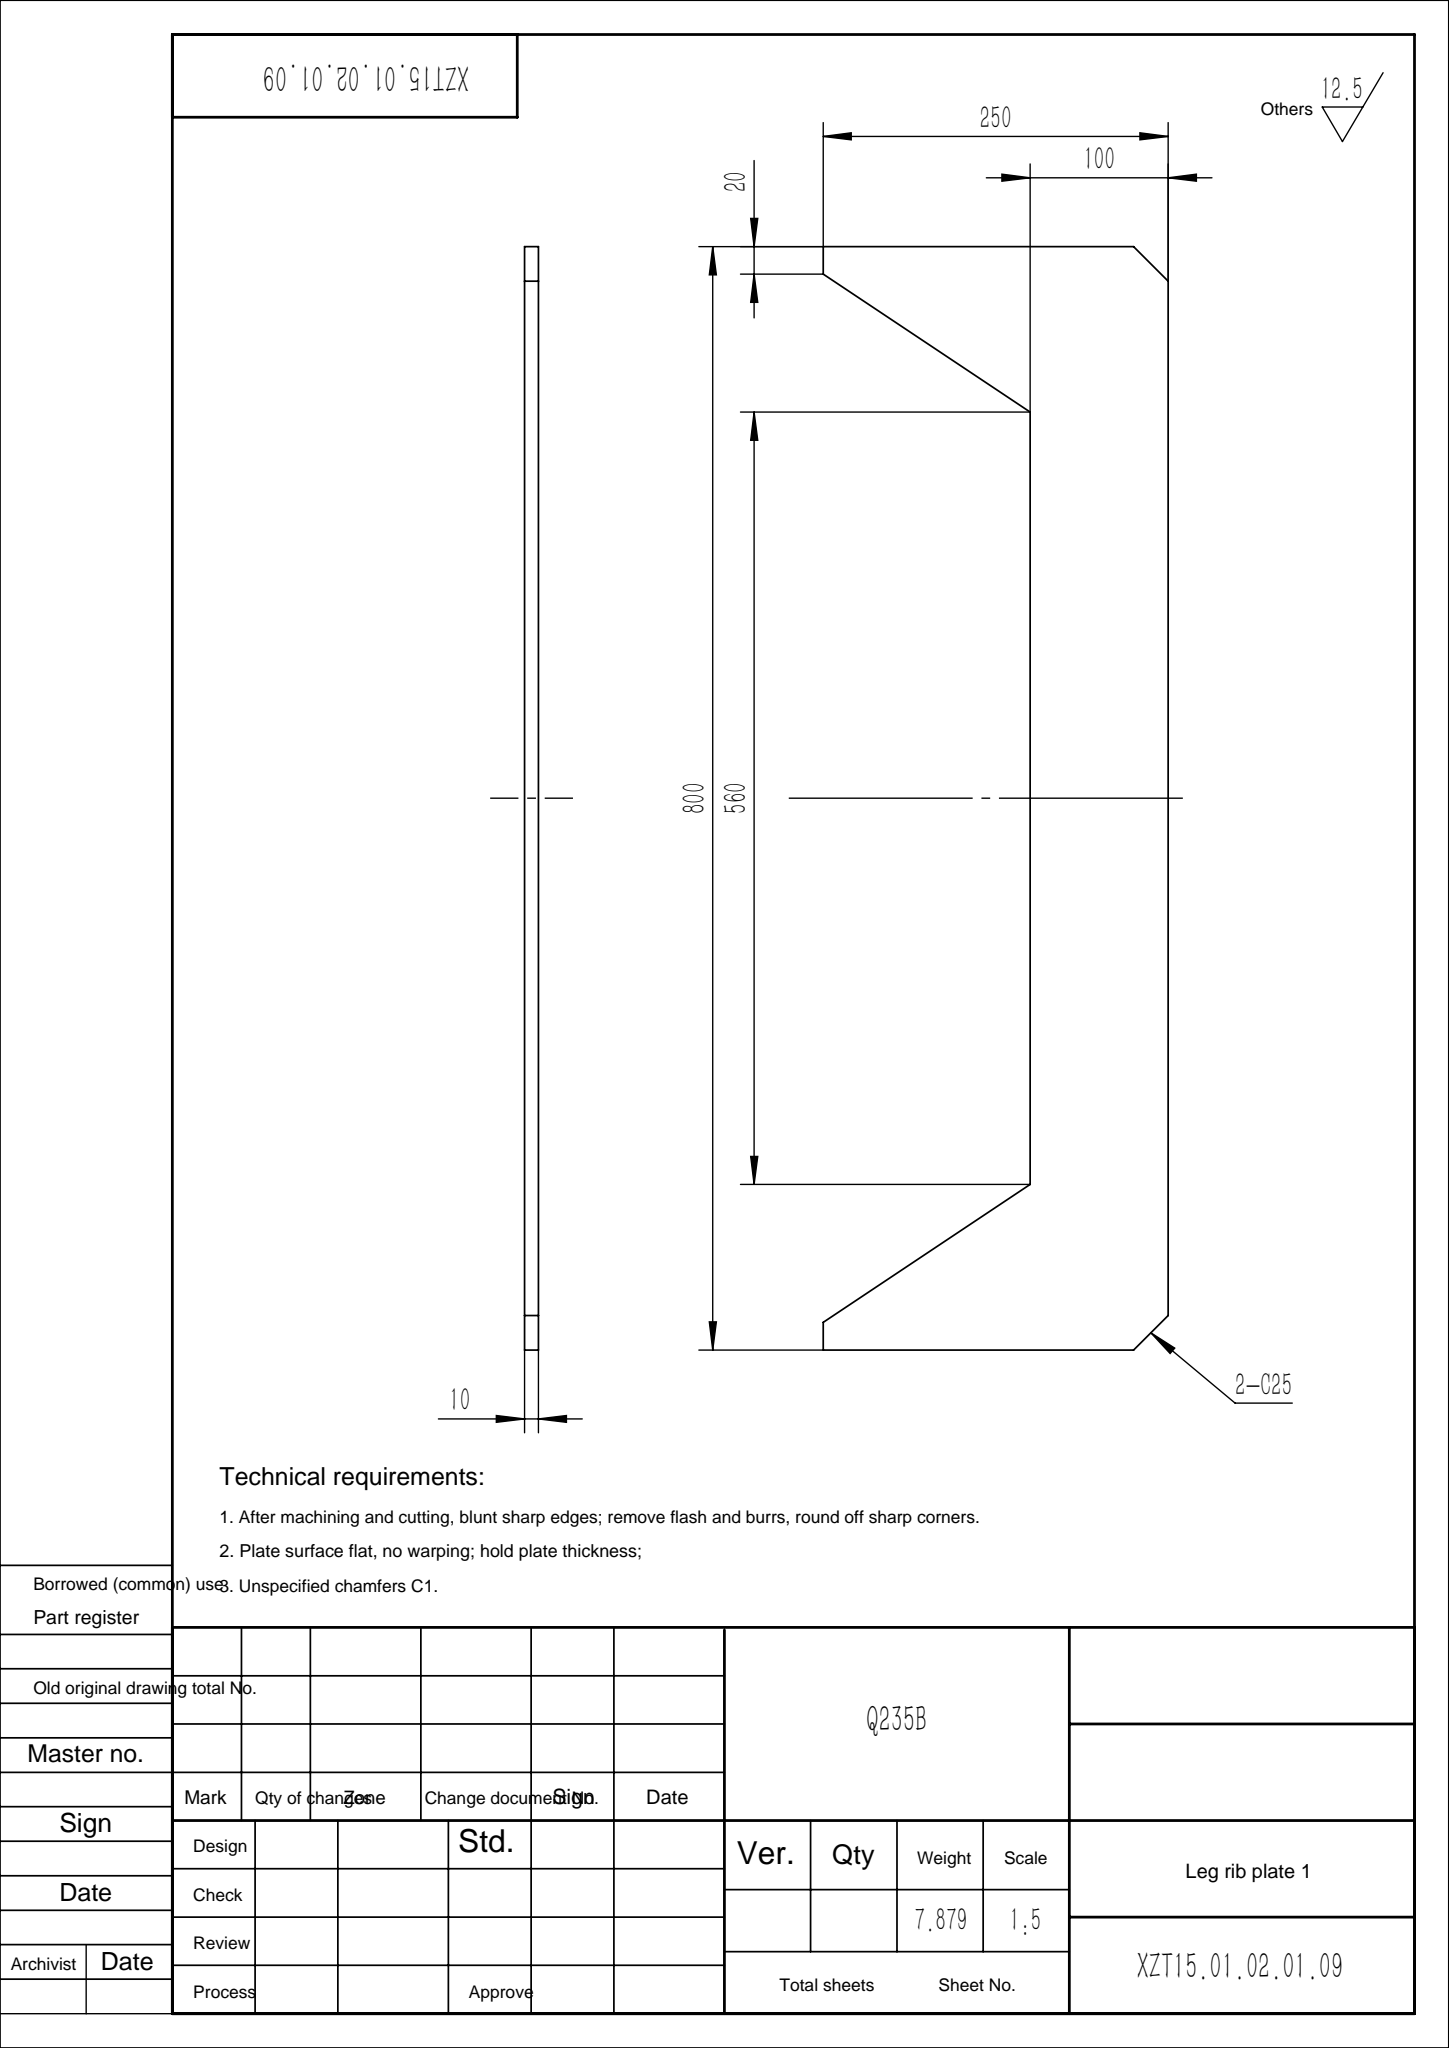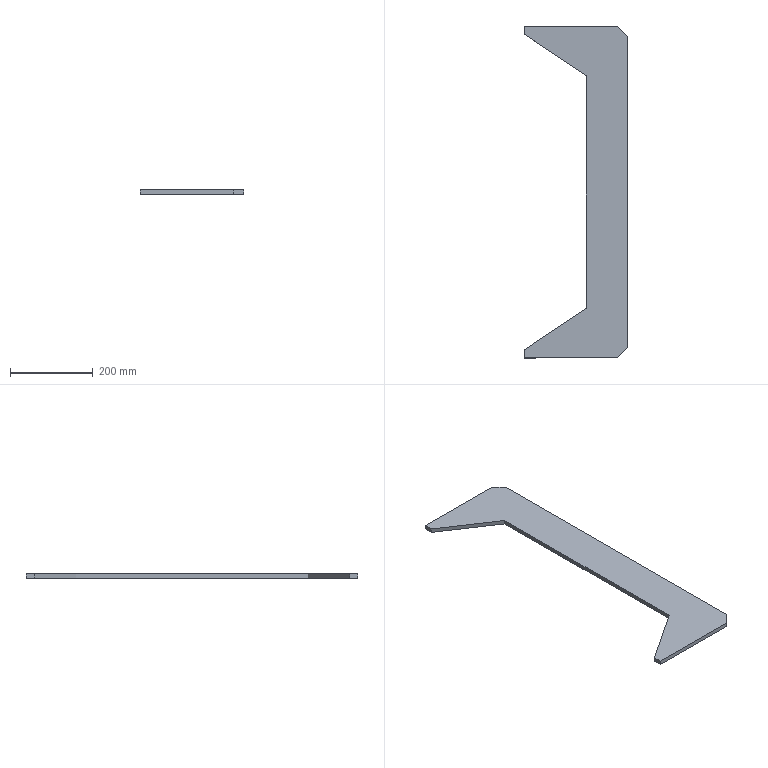Part | SolidWorks | features Chamfer 1, Extrusion 1 | 1 solid | 12 faces | box 250 x 800 x 10 mm | volume 1003750 mm3 | plane 12
STEP:
#1=CARTESIAN_POINT('',(-150.,380.,-5.));
#2=VERTEX_POINT('',#1);
#3=CARTESIAN_POINT('',(0.,280.,-5.));
#4=VERTEX_POINT('',#3);
#5=CARTESIAN_POINT('',(0.,280.,-5.));
#6=DIRECTION('',(0.8321,-0.5547,0.));
#7=VECTOR('',#6,1000.);
#8=LINE('',#5,#7);
#9=EDGE_CURVE('',#2,#4,#8,.T.);
#10=ORIENTED_EDGE('',*,*,#9,.T.);
#11=CARTESIAN_POINT('',(0.,280.,5.));
#12=VERTEX_POINT('',#11);
#13=CARTESIAN_POINT('',(0.,280.,5.));
#14=DIRECTION('',(0.,0.,-1.));
#15=VECTOR('',#14,1000.);
#16=LINE('',#13,#15);
#17=EDGE_CURVE('',#12,#4,#16,.T.);
#18=ORIENTED_EDGE('',*,*,#17,.F.);
#19=CARTESIAN_POINT('',(-150.,380.,5.));
#20=VERTEX_POINT('',#19);
#21=CARTESIAN_POINT('',(0.,280.,5.));
#22=DIRECTION('',(0.8321,-0.5547,0.));
#23=VECTOR('',#22,1000.);
#24=LINE('',#21,#23);
#25=EDGE_CURVE('',#20,#12,#24,.T.);
#26=ORIENTED_EDGE('',*,*,#25,.F.);
#27=CARTESIAN_POINT('',(-150.,380.,5.));
#28=DIRECTION('',(0.,0.,-1.));
#29=VECTOR('',#28,1000.);
#30=LINE('',#27,#29);
#31=EDGE_CURVE('',#20,#2,#30,.T.);
#32=ORIENTED_EDGE('',*,*,#31,.T.);
#33=EDGE_LOOP('',(#10,#18,#26,#32));
#34=FACE_OUTER_BOUND('',#33,.T.);
#35=CARTESIAN_POINT('',(0.,280.,5.));
#36=DIRECTION('',(0.5547,0.8321,0.));
#37=DIRECTION('',(-0.8321,0.5547,0.));
#38=AXIS2_PLACEMENT_3D('',#35,#36,#37);
#39=PLANE('',#38);
#40=ADVANCED_FACE('',(#34),#39,.F.);
#41=CARTESIAN_POINT('',(0.,-280.,-5.));
#42=VERTEX_POINT('',#41);
#43=CARTESIAN_POINT('',(0.,-280.,-5.));
#44=DIRECTION('',(0.,-1.,0.));
#45=VECTOR('',#44,1000.);
#46=LINE('',#43,#45);
#47=EDGE_CURVE('',#4,#42,#46,.T.);
#48=ORIENTED_EDGE('',*,*,#47,.T.);
#49=CARTESIAN_POINT('',(0.,-280.,5.));
#50=VERTEX_POINT('',#49);
#51=CARTESIAN_POINT('',(0.,-280.,5.));
#52=DIRECTION('',(0.,0.,-1.));
#53=VECTOR('',#52,1000.);
#54=LINE('',#51,#53);
#55=EDGE_CURVE('',#50,#42,#54,.T.);
#56=ORIENTED_EDGE('',*,*,#55,.F.);
#57=CARTESIAN_POINT('',(0.,-280.,5.));
#58=DIRECTION('',(0.,-1.,0.));
#59=VECTOR('',#58,1000.);
#60=LINE('',#57,#59);
#61=EDGE_CURVE('',#12,#50,#60,.T.);
#62=ORIENTED_EDGE('',*,*,#61,.F.);
#63=ORIENTED_EDGE('',*,*,#17,.T.);
#64=EDGE_LOOP('',(#48,#56,#62,#63));
#65=FACE_OUTER_BOUND('',#64,.T.);
#66=CARTESIAN_POINT('',(0.,-280.,5.));
#67=DIRECTION('',(1.,0.,0.));
#68=DIRECTION('',(0.,1.,0.));
#69=AXIS2_PLACEMENT_3D('',#66,#67,#68);
#70=PLANE('',#69);
#71=ADVANCED_FACE('',(#65),#70,.F.);
#72=CARTESIAN_POINT('',(-150.,-380.,-5.));
#73=VERTEX_POINT('',#72);
#74=CARTESIAN_POINT('',(0.,-280.,-5.));
#75=DIRECTION('',(-0.8321,-0.5547,0.));
#76=VECTOR('',#75,1000.);
#77=LINE('',#74,#76);
#78=EDGE_CURVE('',#42,#73,#77,.T.);
#79=ORIENTED_EDGE('',*,*,#78,.T.);
#80=CARTESIAN_POINT('',(-150.,-380.,5.));
#81=VERTEX_POINT('',#80);
#82=CARTESIAN_POINT('',(-150.,-380.,5.));
#83=DIRECTION('',(0.,0.,-1.));
#84=VECTOR('',#83,1000.);
#85=LINE('',#82,#84);
#86=EDGE_CURVE('',#81,#73,#85,.T.);
#87=ORIENTED_EDGE('',*,*,#86,.F.);
#88=CARTESIAN_POINT('',(0.,-280.,5.));
#89=DIRECTION('',(-0.8321,-0.5547,0.));
#90=VECTOR('',#89,1000.);
#91=LINE('',#88,#90);
#92=EDGE_CURVE('',#50,#81,#91,.T.);
#93=ORIENTED_EDGE('',*,*,#92,.F.);
#94=ORIENTED_EDGE('',*,*,#55,.T.);
#95=EDGE_LOOP('',(#79,#87,#93,#94));
#96=FACE_OUTER_BOUND('',#95,.T.);
#97=CARTESIAN_POINT('',(0.,-280.,5.));
#98=DIRECTION('',(0.5547,-0.8321,0.));
#99=DIRECTION('',(0.8321,0.5547,0.));
#100=AXIS2_PLACEMENT_3D('',#97,#98,#99);
#101=PLANE('',#100);
#102=ADVANCED_FACE('',(#96),#101,.F.);
#103=CARTESIAN_POINT('',(-150.,-400.,-5.));
#104=VERTEX_POINT('',#103);
#105=CARTESIAN_POINT('',(-150.,-380.,-5.));
#106=DIRECTION('',(0.,-1.,0.));
#107=VECTOR('',#106,1000.);
#108=LINE('',#105,#107);
#109=EDGE_CURVE('',#73,#104,#108,.T.);
#110=ORIENTED_EDGE('',*,*,#109,.T.);
#111=CARTESIAN_POINT('',(-150.,-400.,5.));
#112=VERTEX_POINT('',#111);
#113=CARTESIAN_POINT('',(-150.,-400.,5.));
#114=DIRECTION('',(0.,0.,-1.));
#115=VECTOR('',#114,1000.);
#116=LINE('',#113,#115);
#117=EDGE_CURVE('',#112,#104,#116,.T.);
#118=ORIENTED_EDGE('',*,*,#117,.F.);
#119=CARTESIAN_POINT('',(-150.,-380.,5.));
#120=DIRECTION('',(0.,-1.,0.));
#121=VECTOR('',#120,1000.);
#122=LINE('',#119,#121);
#123=EDGE_CURVE('',#81,#112,#122,.T.);
#124=ORIENTED_EDGE('',*,*,#123,.F.);
#125=ORIENTED_EDGE('',*,*,#86,.T.);
#126=EDGE_LOOP('',(#110,#118,#124,#125));
#127=FACE_OUTER_BOUND('',#126,.T.);
#128=CARTESIAN_POINT('',(-150.,-380.,5.));
#129=DIRECTION('',(1.,0.,0.));
#130=DIRECTION('',(0.,1.,0.));
#131=AXIS2_PLACEMENT_3D('',#128,#129,#130);
#132=PLANE('',#131);
#133=ADVANCED_FACE('',(#127),#132,.F.);
#134=CARTESIAN_POINT('',(75.,-400.,-5.));
#135=VERTEX_POINT('',#134);
#136=CARTESIAN_POINT('',(-150.,-400.,-5.));
#137=DIRECTION('',(1.,0.,0.));
#138=VECTOR('',#137,1000.);
#139=LINE('',#136,#138);
#140=EDGE_CURVE('',#104,#135,#139,.T.);
#141=ORIENTED_EDGE('',*,*,#140,.T.);
#142=CARTESIAN_POINT('',(75.,-400.,5.));
#143=VERTEX_POINT('',#142);
#144=CARTESIAN_POINT('',(75.,-400.,5.));
#145=DIRECTION('',(0.,0.,1.));
#146=VECTOR('',#145,1000.);
#147=LINE('',#144,#146);
#148=EDGE_CURVE('',#135,#143,#147,.T.);
#149=ORIENTED_EDGE('',*,*,#148,.T.);
#150=CARTESIAN_POINT('',(-150.,-400.,5.));
#151=DIRECTION('',(1.,0.,0.));
#152=VECTOR('',#151,1000.);
#153=LINE('',#150,#152);
#154=EDGE_CURVE('',#112,#143,#153,.T.);
#155=ORIENTED_EDGE('',*,*,#154,.F.);
#156=ORIENTED_EDGE('',*,*,#117,.T.);
#157=EDGE_LOOP('',(#141,#149,#155,#156));
#158=FACE_OUTER_BOUND('',#157,.T.);
#159=CARTESIAN_POINT('',(-150.,-400.,5.));
#160=DIRECTION('',(0.,1.,0.));
#161=DIRECTION('',(-1.,0.,0.));
#162=AXIS2_PLACEMENT_3D('',#159,#160,#161);
#163=PLANE('',#162);
#164=ADVANCED_FACE('',(#158),#163,.F.);
#165=CARTESIAN_POINT('',(100.,-375.,5.));
#166=VERTEX_POINT('',#165);
#167=CARTESIAN_POINT('',(100.,375.,5.));
#168=VERTEX_POINT('',#167);
#169=CARTESIAN_POINT('',(100.,400.,5.));
#170=DIRECTION('',(0.,1.,0.));
#171=VECTOR('',#170,1000.);
#172=LINE('',#169,#171);
#173=EDGE_CURVE('',#166,#168,#172,.T.);
#174=ORIENTED_EDGE('',*,*,#173,.F.);
#175=CARTESIAN_POINT('',(100.,-375.,-5.));
#176=VERTEX_POINT('',#175);
#177=CARTESIAN_POINT('',(100.,-375.,5.));
#178=DIRECTION('',(0.,0.,-1.));
#179=VECTOR('',#178,1000.);
#180=LINE('',#177,#179);
#181=EDGE_CURVE('',#166,#176,#180,.T.);
#182=ORIENTED_EDGE('',*,*,#181,.T.);
#183=CARTESIAN_POINT('',(100.,375.,-5.));
#184=VERTEX_POINT('',#183);
#185=CARTESIAN_POINT('',(100.,400.,-5.));
#186=DIRECTION('',(0.,1.,0.));
#187=VECTOR('',#186,1000.);
#188=LINE('',#185,#187);
#189=EDGE_CURVE('',#176,#184,#188,.T.);
#190=ORIENTED_EDGE('',*,*,#189,.T.);
#191=CARTESIAN_POINT('',(100.,375.,5.));
#192=DIRECTION('',(0.,0.,1.));
#193=VECTOR('',#192,1000.);
#194=LINE('',#191,#193);
#195=EDGE_CURVE('',#184,#168,#194,.T.);
#196=ORIENTED_EDGE('',*,*,#195,.T.);
#197=EDGE_LOOP('',(#174,#182,#190,#196));
#198=FACE_OUTER_BOUND('',#197,.T.);
#199=CARTESIAN_POINT('',(100.,400.,5.));
#200=DIRECTION('',(-1.,0.,0.));
#201=DIRECTION('',(0.,-1.,0.));
#202=AXIS2_PLACEMENT_3D('',#199,#200,#201);
#203=PLANE('',#202);
#204=ADVANCED_FACE('',(#198),#203,.F.);
#205=CARTESIAN_POINT('',(75.,400.,5.));
#206=VERTEX_POINT('',#205);
#207=CARTESIAN_POINT('',(-150.,400.,5.));
#208=VERTEX_POINT('',#207);
#209=CARTESIAN_POINT('',(-150.,400.,5.));
#210=DIRECTION('',(-1.,0.,0.));
#211=VECTOR('',#210,1000.);
#212=LINE('',#209,#211);
#213=EDGE_CURVE('',#206,#208,#212,.T.);
#214=ORIENTED_EDGE('',*,*,#213,.F.);
#215=CARTESIAN_POINT('',(75.,400.,-5.));
#216=VERTEX_POINT('',#215);
#217=CARTESIAN_POINT('',(75.,400.,5.));
#218=DIRECTION('',(0.,0.,-1.));
#219=VECTOR('',#218,1000.);
#220=LINE('',#217,#219);
#221=EDGE_CURVE('',#206,#216,#220,.T.);
#222=ORIENTED_EDGE('',*,*,#221,.T.);
#223=CARTESIAN_POINT('',(-150.,400.,-5.));
#224=VERTEX_POINT('',#223);
#225=CARTESIAN_POINT('',(-150.,400.,-5.));
#226=DIRECTION('',(-1.,0.,0.));
#227=VECTOR('',#226,1000.);
#228=LINE('',#225,#227);
#229=EDGE_CURVE('',#216,#224,#228,.T.);
#230=ORIENTED_EDGE('',*,*,#229,.T.);
#231=CARTESIAN_POINT('',(-150.,400.,5.));
#232=DIRECTION('',(0.,0.,-1.));
#233=VECTOR('',#232,1000.);
#234=LINE('',#231,#233);
#235=EDGE_CURVE('',#208,#224,#234,.T.);
#236=ORIENTED_EDGE('',*,*,#235,.F.);
#237=EDGE_LOOP('',(#214,#222,#230,#236));
#238=FACE_OUTER_BOUND('',#237,.T.);
#239=CARTESIAN_POINT('',(-150.,400.,5.));
#240=DIRECTION('',(0.,-1.,0.));
#241=DIRECTION('',(0.,0.,-1.));
#242=AXIS2_PLACEMENT_3D('',#239,#240,#241);
#243=PLANE('',#242);
#244=ADVANCED_FACE('',(#238),#243,.F.);
#245=CARTESIAN_POINT('',(-150.,380.,-5.));
#246=DIRECTION('',(0.,-1.,0.));
#247=VECTOR('',#246,1000.);
#248=LINE('',#245,#247);
#249=EDGE_CURVE('',#224,#2,#248,.T.);
#250=ORIENTED_EDGE('',*,*,#249,.T.);
#251=ORIENTED_EDGE('',*,*,#31,.F.);
#252=CARTESIAN_POINT('',(-150.,380.,5.));
#253=DIRECTION('',(0.,-1.,0.));
#254=VECTOR('',#253,1000.);
#255=LINE('',#252,#254);
#256=EDGE_CURVE('',#208,#20,#255,.T.);
#257=ORIENTED_EDGE('',*,*,#256,.F.);
#258=ORIENTED_EDGE('',*,*,#235,.T.);
#259=EDGE_LOOP('',(#250,#251,#257,#258));
#260=FACE_OUTER_BOUND('',#259,.T.);
#261=CARTESIAN_POINT('',(-150.,380.,5.));
#262=DIRECTION('',(1.,0.,0.));
#263=DIRECTION('',(0.,0.,-1.));
#264=AXIS2_PLACEMENT_3D('',#261,#262,#263);
#265=PLANE('',#264);
#266=ADVANCED_FACE('',(#260),#265,.F.);
#267=ORIENTED_EDGE('',*,*,#154,.T.);
#268=CARTESIAN_POINT('',(237.5,-237.5,5.));
#269=DIRECTION('',(0.7071,0.7071,0.));
#270=VECTOR('',#269,1000.);
#271=LINE('',#268,#270);
#272=EDGE_CURVE('',#143,#166,#271,.T.);
#273=ORIENTED_EDGE('',*,*,#272,.T.);
#274=ORIENTED_EDGE('',*,*,#173,.T.);
#275=CARTESIAN_POINT('',(237.5,237.5,5.));
#276=DIRECTION('',(-0.7071,0.7071,0.));
#277=VECTOR('',#276,1000.);
#278=LINE('',#275,#277);
#279=EDGE_CURVE('',#168,#206,#278,.T.);
#280=ORIENTED_EDGE('',*,*,#279,.T.);
#281=ORIENTED_EDGE('',*,*,#213,.T.);
#282=ORIENTED_EDGE('',*,*,#256,.T.);
#283=ORIENTED_EDGE('',*,*,#25,.T.);
#284=ORIENTED_EDGE('',*,*,#61,.T.);
#285=ORIENTED_EDGE('',*,*,#92,.T.);
#286=ORIENTED_EDGE('',*,*,#123,.T.);
#287=EDGE_LOOP('',(#267,#273,#274,#280,#281,#282,#283,#284,#285,#286));
#288=FACE_OUTER_BOUND('',#287,.T.);
#289=CARTESIAN_POINT('',(0.,0.,5.));
#290=DIRECTION('',(0.,0.,1.));
#291=DIRECTION('',(1.,0.,0.));
#292=AXIS2_PLACEMENT_3D('',#289,#290,#291);
#293=PLANE('',#292);
#294=ADVANCED_FACE('',(#288),#293,.T.);
#295=ORIENTED_EDGE('',*,*,#189,.F.);
#296=CARTESIAN_POINT('',(100.,-375.,-5.));
#297=DIRECTION('',(-0.7071,-0.7071,0.));
#298=VECTOR('',#297,1000.);
#299=LINE('',#296,#298);
#300=EDGE_CURVE('',#176,#135,#299,.T.);
#301=ORIENTED_EDGE('',*,*,#300,.T.);
#302=ORIENTED_EDGE('',*,*,#140,.F.);
#303=ORIENTED_EDGE('',*,*,#109,.F.);
#304=ORIENTED_EDGE('',*,*,#78,.F.);
#305=ORIENTED_EDGE('',*,*,#47,.F.);
#306=ORIENTED_EDGE('',*,*,#9,.F.);
#307=ORIENTED_EDGE('',*,*,#249,.F.);
#308=ORIENTED_EDGE('',*,*,#229,.F.);
#309=CARTESIAN_POINT('',(75.,400.,-5.));
#310=DIRECTION('',(0.7071,-0.7071,0.));
#311=VECTOR('',#310,1000.);
#312=LINE('',#309,#311);
#313=EDGE_CURVE('',#216,#184,#312,.T.);
#314=ORIENTED_EDGE('',*,*,#313,.T.);
#315=EDGE_LOOP('',(#295,#301,#302,#303,#304,#305,#306,#307,#308,#314));
#316=FACE_OUTER_BOUND('',#315,.T.);
#317=CARTESIAN_POINT('',(0.,0.,-5.));
#318=DIRECTION('',(0.,0.,1.));
#319=DIRECTION('',(1.,0.,0.));
#320=AXIS2_PLACEMENT_3D('',#317,#318,#319);
#321=PLANE('',#320);
#322=ADVANCED_FACE('',(#316),#321,.F.);
#323=ORIENTED_EDGE('',*,*,#272,.F.);
#324=ORIENTED_EDGE('',*,*,#148,.F.);
#325=ORIENTED_EDGE('',*,*,#300,.F.);
#326=ORIENTED_EDGE('',*,*,#181,.F.);
#327=EDGE_LOOP('',(#323,#324,#325,#326));
#328=FACE_OUTER_BOUND('',#327,.T.);
#329=CARTESIAN_POINT('',(100.,-375.,5.));
#330=DIRECTION('',(-0.7071,0.7071,0.));
#331=DIRECTION('',(0.,0.,-1.));
#332=AXIS2_PLACEMENT_3D('',#329,#330,#331);
#333=PLANE('',#332);
#334=ADVANCED_FACE('',(#328),#333,.F.);
#335=ORIENTED_EDGE('',*,*,#279,.F.);
#336=ORIENTED_EDGE('',*,*,#195,.F.);
#337=ORIENTED_EDGE('',*,*,#313,.F.);
#338=ORIENTED_EDGE('',*,*,#221,.F.);
#339=EDGE_LOOP('',(#335,#336,#337,#338));
#340=FACE_OUTER_BOUND('',#339,.T.);
#341=CARTESIAN_POINT('',(75.,400.,5.));
#342=DIRECTION('',(-0.7071,-0.7071,0.));
#343=DIRECTION('',(0.,0.,-1.));
#344=AXIS2_PLACEMENT_3D('',#341,#342,#343);
#345=PLANE('',#344);
#346=ADVANCED_FACE('',(#340),#345,.F.);
#347=CLOSED_SHELL('',(#40,#71,#102,#133,#164,#204,#244,#266,#294,#322,#334,#346));
#348=MANIFOLD_SOLID_BREP('',#347);
#349=CARTESIAN_POINT('',(0.,0.,0.));
#350=DIRECTION('',(0.,0.,1.));
#351=DIRECTION('',(1.,0.,0.));
#352=AXIS2_PLACEMENT_3D('',#349,#350,#351);
#353=(LENGTH_UNIT()NAMED_UNIT(*)SI_UNIT(.MILLI.,.METRE.));
#354=UNCERTAINTY_MEASURE_WITH_UNIT(LENGTH_MEASURE(0.00001),#353,'','');
#355=(NAMED_UNIT(*)PLANE_ANGLE_UNIT()SI_UNIT($,.RADIAN.));
#356=(NAMED_UNIT(*)SI_UNIT($,.STERADIAN.)SOLID_ANGLE_UNIT());
#357=(GEOMETRIC_REPRESENTATION_CONTEXT(3)GLOBAL_UNCERTAINTY_ASSIGNED_CONTEXT((#354))GLOBAL_UNIT_ASSIGNED_CONTEXT((#353,#355,#356))REPRESENTATION_CONTEXT('',''));
#358=ADVANCED_BREP_SHAPE_REPRESENTATION('',(#348,#352),#357);